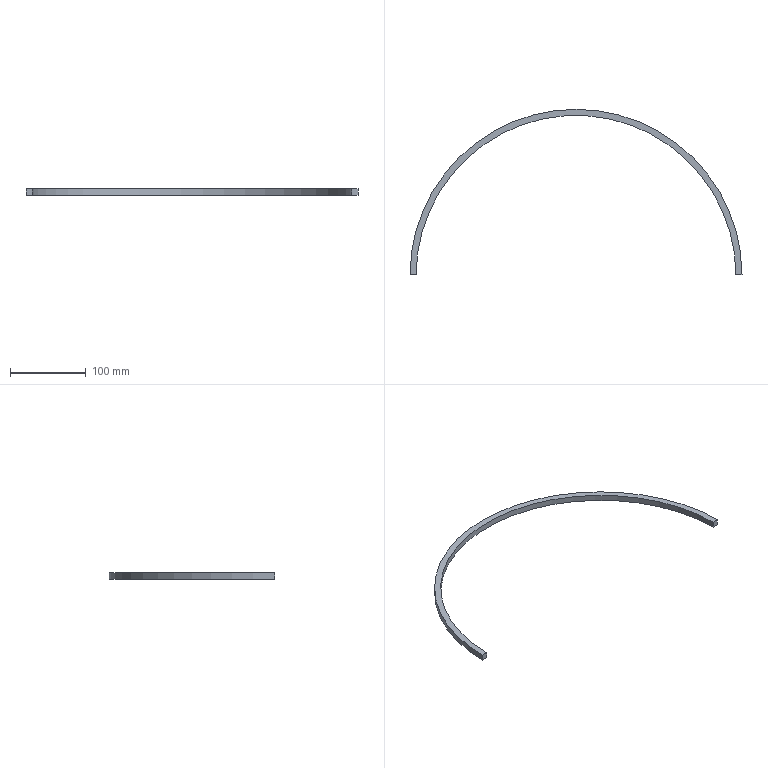Part | SolidWorks | features Extrusion 1 | 1 solid | 6 faces | box 437.995 x 218 x 8 mm | volume 43100 mm3 | plane 4 | cylinder 2 | commonest cylinder face diameters 422 x1 438 x1
STEP:
#1=CARTESIAN_POINT('',(438.998,1.,4.));
#2=VERTEX_POINT('',#1);
#3=CARTESIAN_POINT('',(1.002,1.,4.));
#4=VERTEX_POINT('',#3);
#5=CARTESIAN_POINT('',(220.,0.,4.));
#6=DIRECTION('',(0.,0.,1.));
#7=DIRECTION('',(1.,0.,0.));
#8=AXIS2_PLACEMENT_3D('',#5,#6,#7);
#9=CIRCLE('',#8,219.);
#10=EDGE_CURVE('',#2,#4,#9,.T.);
#11=ORIENTED_EDGE('',*,*,#10,.F.);
#12=CARTESIAN_POINT('',(438.998,1.,-4.));
#13=VERTEX_POINT('',#12);
#14=CARTESIAN_POINT('',(438.998,1.,-4.));
#15=DIRECTION('',(0.,0.,1.));
#16=VECTOR('',#15,1000.);
#17=LINE('',#14,#16);
#18=EDGE_CURVE('',#13,#2,#17,.T.);
#19=ORIENTED_EDGE('',*,*,#18,.F.);
#20=CARTESIAN_POINT('',(1.002,1.,-4.));
#21=VERTEX_POINT('',#20);
#22=CARTESIAN_POINT('',(220.,0.,-4.));
#23=DIRECTION('',(0.,0.,1.));
#24=DIRECTION('',(1.,0.,0.));
#25=AXIS2_PLACEMENT_3D('',#22,#23,#24);
#26=CIRCLE('',#25,219.);
#27=EDGE_CURVE('',#13,#21,#26,.T.);
#28=ORIENTED_EDGE('',*,*,#27,.T.);
#29=CARTESIAN_POINT('',(1.002,1.,-4.));
#30=DIRECTION('',(0.,0.,1.));
#31=VECTOR('',#30,1000.);
#32=LINE('',#29,#31);
#33=EDGE_CURVE('',#21,#4,#32,.T.);
#34=ORIENTED_EDGE('',*,*,#33,.T.);
#35=EDGE_LOOP('',(#11,#19,#28,#34));
#36=FACE_OUTER_BOUND('',#35,.T.);
#37=CARTESIAN_POINT('',(220.,0.,-4.));
#38=DIRECTION('',(0.,0.,1.));
#39=DIRECTION('',(1.,0.,0.));
#40=AXIS2_PLACEMENT_3D('',#37,#38,#39);
#41=CYLINDRICAL_SURFACE('',#40,219.);
#42=ADVANCED_FACE('',(#36),#41,.T.);
#43=CARTESIAN_POINT('',(430.998,1.,4.));
#44=VERTEX_POINT('',#43);
#45=CARTESIAN_POINT('',(430.998,1.,4.));
#46=DIRECTION('',(1.,0.,0.));
#47=VECTOR('',#46,1000.);
#48=LINE('',#45,#47);
#49=EDGE_CURVE('',#44,#2,#48,.T.);
#50=ORIENTED_EDGE('',*,*,#49,.F.);
#51=CARTESIAN_POINT('',(430.998,1.,-4.));
#52=VERTEX_POINT('',#51);
#53=CARTESIAN_POINT('',(430.998,1.,-4.));
#54=DIRECTION('',(0.,0.,1.));
#55=VECTOR('',#54,1000.);
#56=LINE('',#53,#55);
#57=EDGE_CURVE('',#52,#44,#56,.T.);
#58=ORIENTED_EDGE('',*,*,#57,.F.);
#59=CARTESIAN_POINT('',(430.998,1.,-4.));
#60=DIRECTION('',(1.,0.,0.));
#61=VECTOR('',#60,1000.);
#62=LINE('',#59,#61);
#63=EDGE_CURVE('',#52,#13,#62,.T.);
#64=ORIENTED_EDGE('',*,*,#63,.T.);
#65=ORIENTED_EDGE('',*,*,#18,.T.);
#66=EDGE_LOOP('',(#50,#58,#64,#65));
#67=FACE_OUTER_BOUND('',#66,.T.);
#68=CARTESIAN_POINT('',(430.998,1.,-4.));
#69=DIRECTION('',(0.,-1.,0.));
#70=DIRECTION('',(1.,0.,0.));
#71=AXIS2_PLACEMENT_3D('',#68,#69,#70);
#72=PLANE('',#71);
#73=ADVANCED_FACE('',(#67),#72,.T.);
#74=CARTESIAN_POINT('',(9.002,1.,4.));
#75=VERTEX_POINT('',#74);
#76=CARTESIAN_POINT('',(220.,0.,4.));
#77=DIRECTION('',(0.,0.,-1.));
#78=DIRECTION('',(-1.,0.,0.));
#79=AXIS2_PLACEMENT_3D('',#76,#77,#78);
#80=CIRCLE('',#79,211.);
#81=EDGE_CURVE('',#75,#44,#80,.T.);
#82=ORIENTED_EDGE('',*,*,#81,.F.);
#83=CARTESIAN_POINT('',(9.002,1.,-4.));
#84=VERTEX_POINT('',#83);
#85=CARTESIAN_POINT('',(9.002,1.,-4.));
#86=DIRECTION('',(0.,0.,1.));
#87=VECTOR('',#86,1000.);
#88=LINE('',#85,#87);
#89=EDGE_CURVE('',#84,#75,#88,.T.);
#90=ORIENTED_EDGE('',*,*,#89,.F.);
#91=CARTESIAN_POINT('',(220.,0.,-4.));
#92=DIRECTION('',(0.,0.,-1.));
#93=DIRECTION('',(-1.,0.,0.));
#94=AXIS2_PLACEMENT_3D('',#91,#92,#93);
#95=CIRCLE('',#94,211.);
#96=EDGE_CURVE('',#84,#52,#95,.T.);
#97=ORIENTED_EDGE('',*,*,#96,.T.);
#98=ORIENTED_EDGE('',*,*,#57,.T.);
#99=EDGE_LOOP('',(#82,#90,#97,#98));
#100=FACE_OUTER_BOUND('',#99,.T.);
#101=CARTESIAN_POINT('',(220.,0.,-4.));
#102=DIRECTION('',(0.,0.,1.));
#103=DIRECTION('',(1.,0.,0.));
#104=AXIS2_PLACEMENT_3D('',#101,#102,#103);
#105=CYLINDRICAL_SURFACE('',#104,211.);
#106=ADVANCED_FACE('',(#100),#105,.F.);
#107=CARTESIAN_POINT('',(1.002,1.,4.));
#108=DIRECTION('',(1.,0.,0.));
#109=VECTOR('',#108,1000.);
#110=LINE('',#107,#109);
#111=EDGE_CURVE('',#4,#75,#110,.T.);
#112=ORIENTED_EDGE('',*,*,#111,.F.);
#113=ORIENTED_EDGE('',*,*,#33,.F.);
#114=CARTESIAN_POINT('',(1.002,1.,-4.));
#115=DIRECTION('',(1.,0.,0.));
#116=VECTOR('',#115,1000.);
#117=LINE('',#114,#116);
#118=EDGE_CURVE('',#21,#84,#117,.T.);
#119=ORIENTED_EDGE('',*,*,#118,.T.);
#120=ORIENTED_EDGE('',*,*,#89,.T.);
#121=EDGE_LOOP('',(#112,#113,#119,#120));
#122=FACE_OUTER_BOUND('',#121,.T.);
#123=CARTESIAN_POINT('',(1.002,1.,-4.));
#124=DIRECTION('',(0.,-1.,0.));
#125=DIRECTION('',(1.,0.,0.));
#126=AXIS2_PLACEMENT_3D('',#123,#124,#125);
#127=PLANE('',#126);
#128=ADVANCED_FACE('',(#122),#127,.T.);
#129=ORIENTED_EDGE('',*,*,#27,.F.);
#130=ORIENTED_EDGE('',*,*,#63,.F.);
#131=ORIENTED_EDGE('',*,*,#96,.F.);
#132=ORIENTED_EDGE('',*,*,#118,.F.);
#133=EDGE_LOOP('',(#129,#130,#131,#132));
#134=FACE_OUTER_BOUND('',#133,.T.);
#135=CARTESIAN_POINT('',(220.,0.,-4.));
#136=DIRECTION('',(0.,0.,1.));
#137=DIRECTION('',(1.,0.,0.));
#138=AXIS2_PLACEMENT_3D('',#135,#136,#137);
#139=PLANE('',#138);
#140=ADVANCED_FACE('',(#134),#139,.F.);
#141=ORIENTED_EDGE('',*,*,#10,.T.);
#142=ORIENTED_EDGE('',*,*,#111,.T.);
#143=ORIENTED_EDGE('',*,*,#81,.T.);
#144=ORIENTED_EDGE('',*,*,#49,.T.);
#145=EDGE_LOOP('',(#141,#142,#143,#144));
#146=FACE_OUTER_BOUND('',#145,.T.);
#147=CARTESIAN_POINT('',(220.,0.,4.));
#148=DIRECTION('',(0.,0.,1.));
#149=DIRECTION('',(1.,0.,0.));
#150=AXIS2_PLACEMENT_3D('',#147,#148,#149);
#151=PLANE('',#150);
#152=ADVANCED_FACE('',(#146),#151,.T.);
#153=CLOSED_SHELL('',(#42,#73,#106,#128,#140,#152));
#154=MANIFOLD_SOLID_BREP('',#153);
#155=CARTESIAN_POINT('',(0.,0.,0.));
#156=DIRECTION('',(0.,0.,1.));
#157=DIRECTION('',(1.,0.,0.));
#158=AXIS2_PLACEMENT_3D('',#155,#156,#157);
#159=(LENGTH_UNIT()NAMED_UNIT(*)SI_UNIT(.MILLI.,.METRE.));
#160=UNCERTAINTY_MEASURE_WITH_UNIT(LENGTH_MEASURE(0.00001),#159,'','');
#161=(NAMED_UNIT(*)PLANE_ANGLE_UNIT()SI_UNIT($,.RADIAN.));
#162=(NAMED_UNIT(*)SI_UNIT($,.STERADIAN.)SOLID_ANGLE_UNIT());
#163=(GEOMETRIC_REPRESENTATION_CONTEXT(3)GLOBAL_UNCERTAINTY_ASSIGNED_CONTEXT((#160))GLOBAL_UNIT_ASSIGNED_CONTEXT((#159,#161,#162))REPRESENTATION_CONTEXT('',''));
#164=ADVANCED_BREP_SHAPE_REPRESENTATION('',(#154,#158),#163);